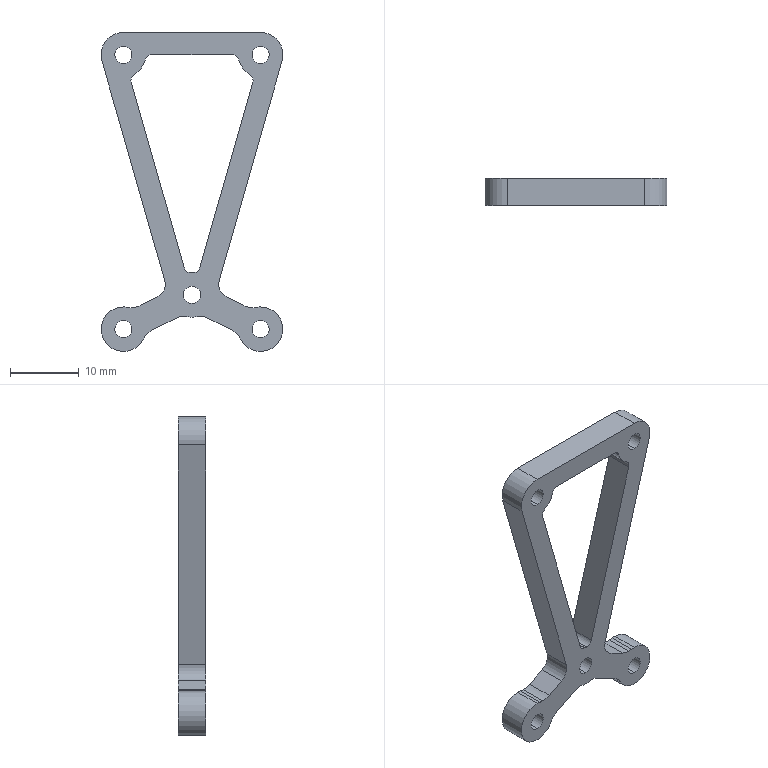Part | SolidWorks | features Fillet 3, Extrusion 1 | 1 solid | 53 faces | box 26.5 x 4 x 46.5 mm | volume 1746 mm3 | cylinder 41 | plane 12 | commonest cylinder face diameters 6.5 x13 2.5 x10 2 x8 6 x6 4 x4